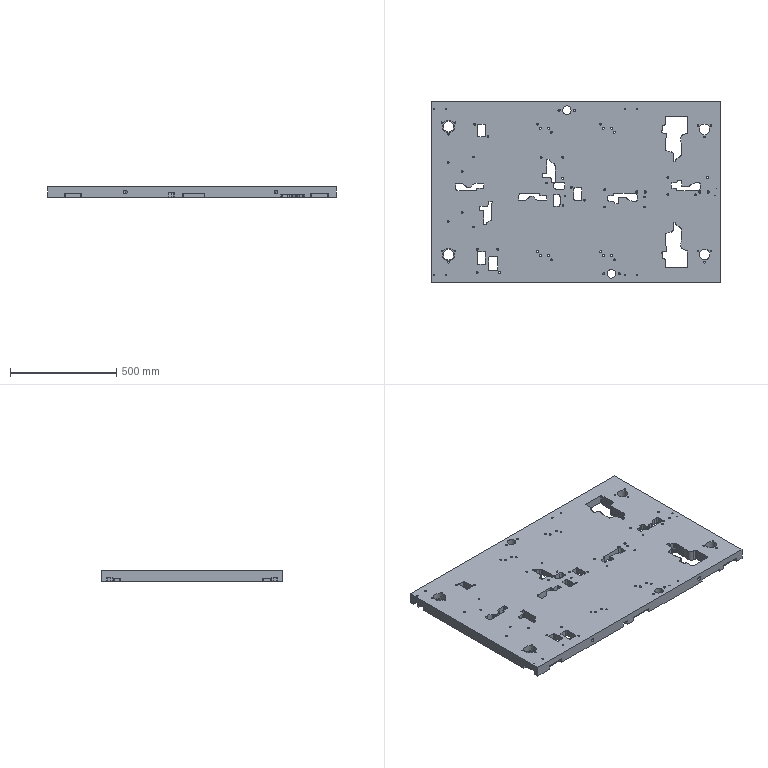Part | STEP file | lll_id18_x_t | 1 solid | 804 faces | box 1360 x 850 x 50 mm | volume 49252374 mm3 | cylinder 477 | plane 293 | cone 34 | commonest cylinder face diameters 10 x101 8.506 x30 7 x28 5 x20 8 x18 20 x17